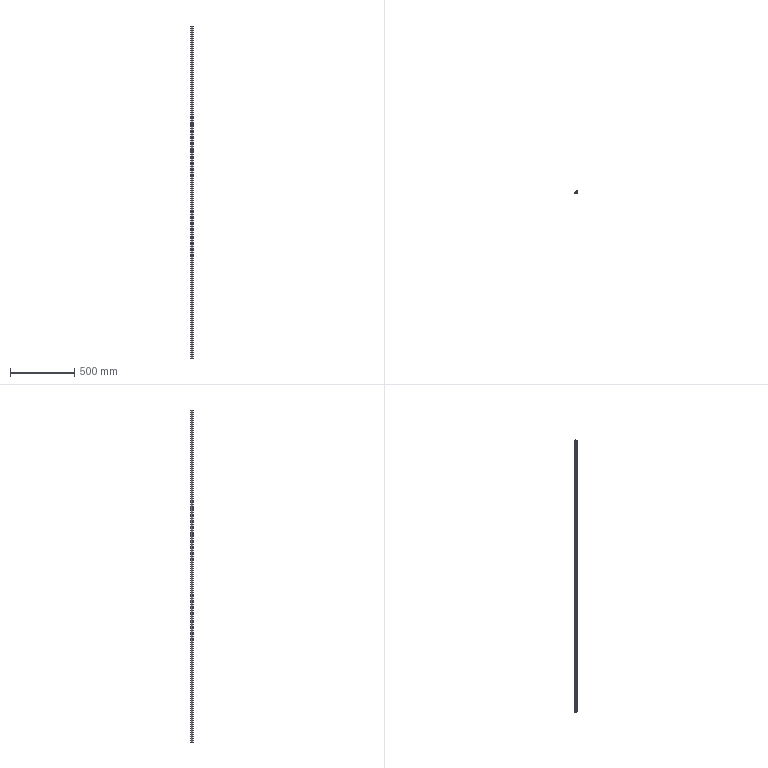Part | 1 solid | 50 faces | box 20 x 16 x 2576 mm | volume 284041 mm3 | plane 35 | cylinder 15 | commonest cylinder face diameters 0.6 x10 0.4 x3 4 x2